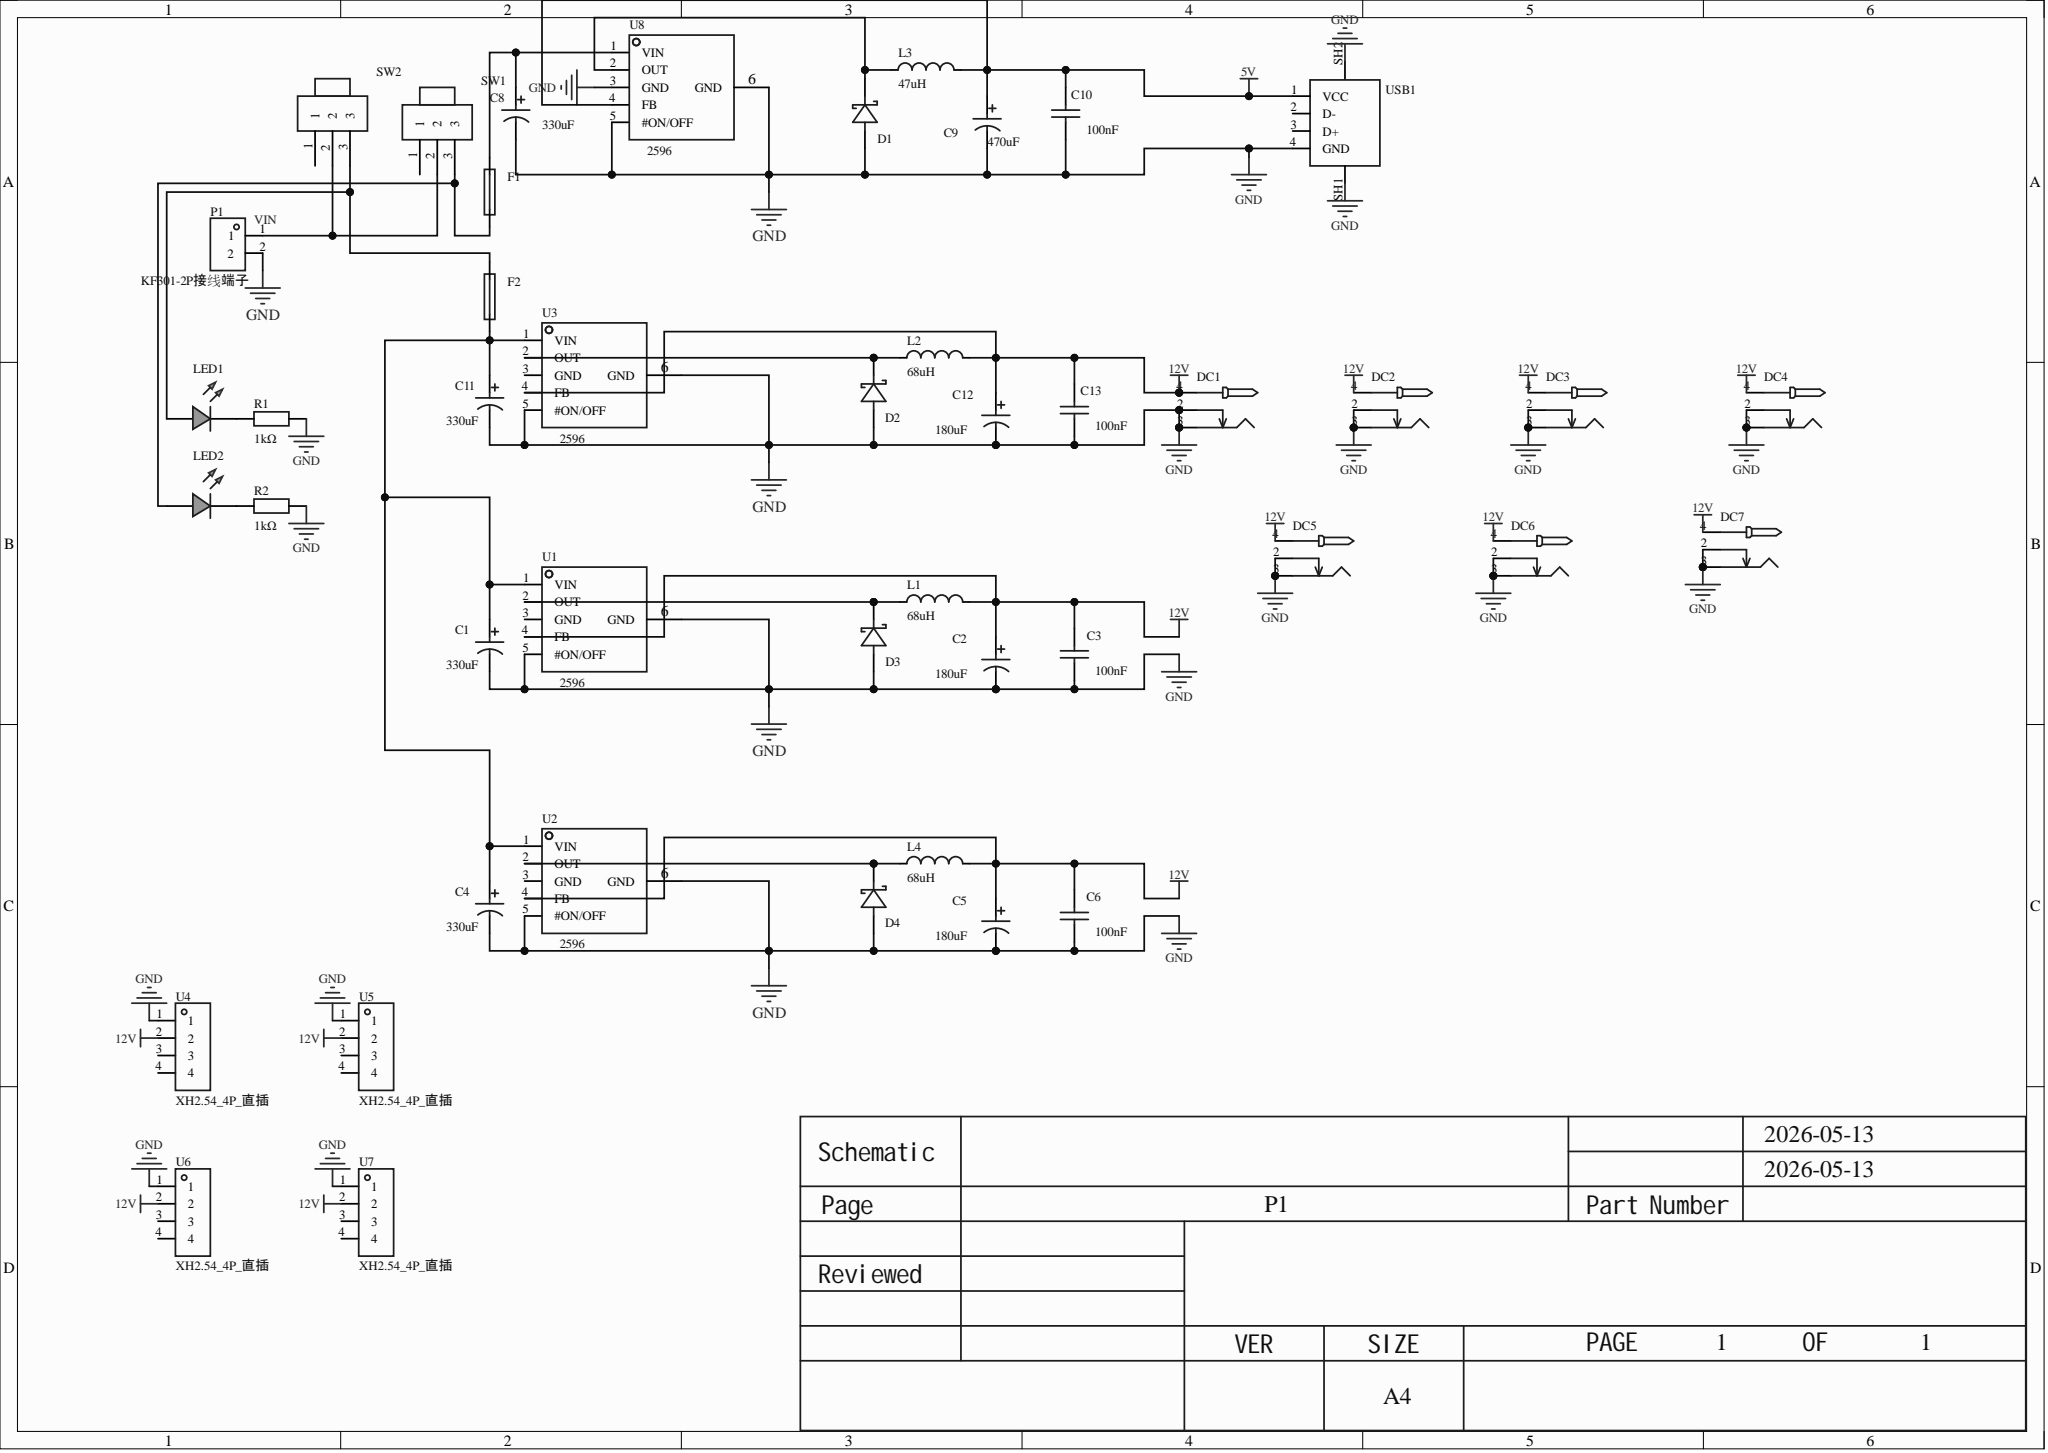Circuit board | Altium Designer | 45 parts | 14 nets
Bill of materials:
Comment,Description,Designator,Footprint,LibRef,Quantity
"","","C1, C2, C4, C5, C8, C9, C11, C12","CAP-SMD_BD8.0-L8.3-W8.3-RD","CS1V221M-CRF10","8"
"","","C3, C6, C10, C13","C0805","CL21B104KBCNNNC","4"
"","","D1, D2, D3, D4","SMA_L4.3-W2.6-LS5.2-RD","SS34_3","4"
"","","DC1, DC2, DC3, DC4, DC5, DC6, DC7","DC-2.0","DC-005_2.0","7"
"10A保险丝","","F1, F2","FUSE-SMD_L6.1-W2.6","10A保险丝","2"
"","","L1, L2, L3, L4","IND-SMD_L7.0-W6.6","CMLO0630H330MTT","4"
"","","LED1, LED2","LED_TH-3mm","LED_TH-G_3mm","2"
"KF301-2P接线端子","","P1","CONN-TH_XY301V-A-5.0-2P","KF301-2P接线端子","1"
"1kΩ","","R1, R2","Res_1/8W","Res_AXIAL-1/8W","2"
"船型开关601-10211BB","","SW1, SW2","SW-TH_601-10211BB","船型开关601-10211BB","2"
"LM2596S-12","","U1, U2, U3","TO-263-5_L10.0-W8.4-P1.70-LS15.3-BR","LM2596S-12_C347422","3"
"XH2.54_4P_直插","","U4, U5, U6, U7","CONN-TH_4P-P2.50-XH2.54-4P","XH2.54_4P_直插","4"
"LM2596S-5.0","","U8","TO-263-5_L10.2-W8.9-P1.70-BR","LM2596S-5.0_C347421","1"
"","","USB1","USB_ Type-A","USB_ Type-A","1"
Netlist (Protel format):
[
C1
CAP-SMD_BD8.0-L8.3-W8.3-RD




]
[
C2
CAP-SMD_BD8.0-L8.3-W8.3-RD




]
[
C3
C0805




]
[
C4
CAP-SMD_BD8.0-L8.3-W8.3-RD




]
[
C5
CAP-SMD_BD8.0-L8.3-W8.3-RD




]
[
C6
C0805




]
[
C8
CAP-SMD_BD8.0-L8.3-W8.3-RD




]
[
C9
CAP-SMD_BD8.0-L8.3-W8.3-RD




]
[
C10
C0805




]
[
C11
CAP-SMD_BD8.0-L8.3-W8.3-RD




]
[
C12
CAP-SMD_BD8.0-L8.3-W8.3-RD




]
[
C13
C0805




]
[
D1
SMA_L4.3-W2.6-LS5.2-RD




]
[
D2
SMA_L4.3-W2.6-LS5.2-RD




]
[
D3
SMA_L4.3-W2.6-LS5.2-RD




]
[
D4
SMA_L4.3-W2.6-LS5.2-RD




]
[
DC1
DC-2.0




]
[
DC2
DC-2.0




]
[
DC3
DC-2.0




]
[
DC4
DC-2.0




]
[
DC5
DC-2.0




]
[
DC6
DC-2.0




]
[
DC7
DC-2.0




]
[
F1
FUSE-SMD_L6.1-W2.6
10A保险丝



]
[
F2
FUSE-SMD_L6.1-W2.6
10A保险丝



]
[
L1
IND-SMD_L7.0-W6.6




]
[
L2
IND-SMD_L7.0-W6.6




]
[
L3
IND-SMD_L7.0-W6.6




]
[
L4
IND-SMD_L7.0-W6.6




]
[
LED1
LED_TH-3mm




]
[
LED2
LED_TH-3mm




]
[
P1
CONN-TH_XY301V-A-5.0-2P
KF301-2P接线端子



]
[
R1
Res_1/8W
1kΩ



]
[
R2
Res_1/8W
1kΩ



]
[
SW1
SW-TH_601-10211BB
船型开关601-10211BB



]
[
SW2
SW-TH_601-10211BB
船型开关601-10211BB



]
[
U1
TO-263-5_L10.0-W8.4-P1.70-LS15.3-BR
LM2596S-12



]
[
U2
TO-263-5_L10.0-W8.4-P1.70-LS15.3-BR
LM2596S-12



]
[
U3
TO-263-5_L10.0-W8.4-P1.70-LS15.3-BR
LM2596S-12



]
[
U4
CONN-TH_4P-P2.50-XH2.54-4P
XH2.54_4P_直插



]
[
U5
CONN-TH_4P-P2.50-XH2.54-4P
XH2.54_4P_直插



]
[
U6
CONN-TH_4P-P2.50-XH2.54-4P
XH2.54_4P_直插



]
[
U7
CONN-TH_4P-P2.50-XH2.54-4P
XH2.54_4P_直插



]
[
U8
TO-263-5_L10.2-W8.9-P1.70-BR
LM2596S-5.0



]
[
USB1
USB_ Type-A




]
(
NetP1_1
P1-1
SW1-2
SW2-2
)
(
NetLED2_2
LED2-2
R2-1
)
(
NetLED1_2
LED1-2
R1-1
)
(
NetF2_2
F2-2
LED1-1
SW2-3
)
(
NetF1_1
F1-1
LED2-1
SW1-3
)
(
NetD4_1
D4-1
L4-1
U2-2
)
(
NetD3_1
D3-1
L1-1
U1-2
)
(
NetD2_1
D2-1
L2-1
U3-2
)
(
NetD1_1
D1-1
L3-1
U8-2
)
(
NetC8_1
C8-1
F1-2
U8-1
)
(
NetC1_1
C1-1
C4-1
C11-1
F2-1
U1-1
U2-1
U3-1
)
(
GND
C1-2
C2-2
C3-2
C4-2
C5-2
C6-2
C8-2
C9-2
C10-2
C11-2
C12-2
C13-2
D1-2
D2-2
D3-2
D4-2
DC1-2
DC1-3
DC2-2
DC2-3
DC3-2
DC3-3
DC4-2
DC4-3
DC5-2
DC5-3
DC6-2
DC6-3
DC7-2
DC7-3
P1-2
R1-2
R2-2
U1-5
U1-6
U2-5
U2-6
U3-5
U3-6
U4-1
U5-1
U6-1
U7-1
U8-3
U8-5
U8-6
USB1-4
USB1-SH1
USB1-SH2
)
(
12V
C2-1
C3-1
C5-1
C6-1
C12-1
C13-1
DC1-4
DC2-4
DC3-4
DC4-4
DC5-4
DC6-4
DC7-4
L1-2
L2-2
L4-2
U1-4
U2-4
U3-4
U4-2
U5-2
U6-2
U7-2
)
(
5V
C9-1
C10-1
L3-2
U8-4
USB1-1
)